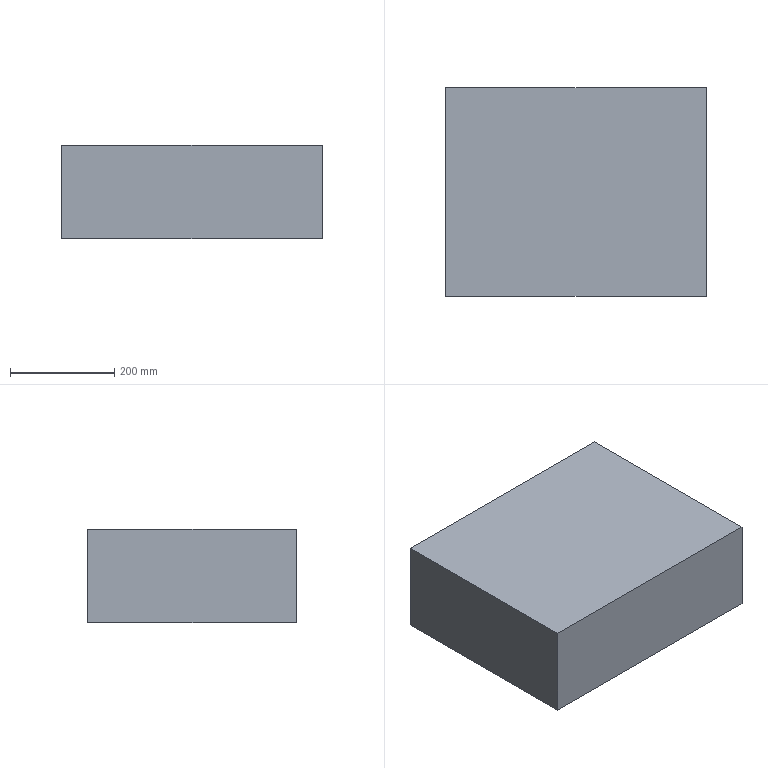Part | NX | features main panel 2 | 1 solid | 6 faces | box 500 x 400 x 180 mm | volume 36000000 mm3 | plane 6
STEP:
#1=CARTESIAN_POINT('',(250.,-600.,0.));
#2=VERTEX_POINT('',#1);
#3=CARTESIAN_POINT('',(-250.,-600.,0.));
#4=VERTEX_POINT('',#3);
#5=CARTESIAN_POINT('',(-250.,-600.,0.));
#6=DIRECTION('',(1.,0.,0.));
#7=VECTOR('',#6,1000.);
#8=LINE('',#5,#7);
#9=EDGE_CURVE('',#2,#4,#8,.F.);
#10=ORIENTED_EDGE('',*,*,#9,.F.);
#11=CARTESIAN_POINT('',(250.,-200.,0.));
#12=VERTEX_POINT('',#11);
#13=CARTESIAN_POINT('',(250.,-600.,0.));
#14=DIRECTION('',(0.,1.,0.));
#15=VECTOR('',#14,1000.);
#16=LINE('',#13,#15);
#17=EDGE_CURVE('',#12,#2,#16,.F.);
#18=ORIENTED_EDGE('',*,*,#17,.F.);
#19=CARTESIAN_POINT('',(-250.,-200.,0.));
#20=VERTEX_POINT('',#19);
#21=CARTESIAN_POINT('',(-250.,-200.,0.));
#22=DIRECTION('',(1.,0.,0.));
#23=VECTOR('',#22,1000.);
#24=LINE('',#21,#23);
#25=EDGE_CURVE('',#20,#12,#24,.T.);
#26=ORIENTED_EDGE('',*,*,#25,.F.);
#27=CARTESIAN_POINT('',(-250.,-600.,0.));
#28=DIRECTION('',(0.,1.,0.));
#29=VECTOR('',#28,1000.);
#30=LINE('',#27,#29);
#31=EDGE_CURVE('',#4,#20,#30,.T.);
#32=ORIENTED_EDGE('',*,*,#31,.F.);
#33=EDGE_LOOP('',(#10,#18,#26,#32));
#34=FACE_BOUND('',#33,.T.);
#35=CARTESIAN_POINT('',(-250.,-200.,0.));
#36=DIRECTION('',(0.,0.,-1.));
#37=DIRECTION('',(-1.,0.,0.));
#38=AXIS2_PLACEMENT_3D('',#35,#36,#37);
#39=PLANE('',#38);
#40=ADVANCED_FACE('',(#34),#39,.F.);
#41=CARTESIAN_POINT('',(-250.,-600.,-180.));
#42=VERTEX_POINT('',#41);
#43=CARTESIAN_POINT('',(-250.,-200.,-180.));
#44=VERTEX_POINT('',#43);
#45=CARTESIAN_POINT('',(-250.,-200.,-180.));
#46=DIRECTION('',(0.,1.,0.));
#47=VECTOR('',#46,1000.);
#48=LINE('',#45,#47);
#49=EDGE_CURVE('',#42,#44,#48,.T.);
#50=ORIENTED_EDGE('',*,*,#49,.F.);
#51=CARTESIAN_POINT('',(-250.,-600.,-180.));
#52=DIRECTION('',(0.,0.,-1.));
#53=VECTOR('',#52,1000.);
#54=LINE('',#51,#53);
#55=EDGE_CURVE('',#4,#42,#54,.T.);
#56=ORIENTED_EDGE('',*,*,#55,.F.);
#57=ORIENTED_EDGE('',*,*,#31,.T.);
#58=CARTESIAN_POINT('',(-250.,-200.,-180.));
#59=DIRECTION('',(0.,0.,1.));
#60=VECTOR('',#59,1000.);
#61=LINE('',#58,#60);
#62=EDGE_CURVE('',#44,#20,#61,.T.);
#63=ORIENTED_EDGE('',*,*,#62,.F.);
#64=EDGE_LOOP('',(#50,#56,#57,#63));
#65=FACE_BOUND('',#64,.T.);
#66=CARTESIAN_POINT('',(-250.,-600.,-180.));
#67=DIRECTION('',(-1.,0.,0.));
#68=DIRECTION('',(0.,0.,1.));
#69=AXIS2_PLACEMENT_3D('',#66,#67,#68);
#70=PLANE('',#69);
#71=ADVANCED_FACE('',(#65),#70,.T.);
#72=CARTESIAN_POINT('',(250.,-200.,-180.));
#73=VERTEX_POINT('',#72);
#74=CARTESIAN_POINT('',(-250.,-200.,-180.));
#75=DIRECTION('',(-1.,0.,0.));
#76=VECTOR('',#75,1000.);
#77=LINE('',#74,#76);
#78=EDGE_CURVE('',#44,#73,#77,.F.);
#79=ORIENTED_EDGE('',*,*,#78,.F.);
#80=ORIENTED_EDGE('',*,*,#62,.T.);
#81=ORIENTED_EDGE('',*,*,#25,.T.);
#82=CARTESIAN_POINT('',(250.,-200.,-180.));
#83=DIRECTION('',(0.,0.,-1.));
#84=VECTOR('',#83,1000.);
#85=LINE('',#82,#84);
#86=EDGE_CURVE('',#73,#12,#85,.F.);
#87=ORIENTED_EDGE('',*,*,#86,.F.);
#88=EDGE_LOOP('',(#79,#80,#81,#87));
#89=FACE_BOUND('',#88,.T.);
#90=CARTESIAN_POINT('',(-250.,-200.,-180.));
#91=DIRECTION('',(0.,1.,0.));
#92=DIRECTION('',(0.,0.,1.));
#93=AXIS2_PLACEMENT_3D('',#90,#91,#92);
#94=PLANE('',#93);
#95=ADVANCED_FACE('',(#89),#94,.T.);
#96=CARTESIAN_POINT('',(250.,-600.,-180.));
#97=VERTEX_POINT('',#96);
#98=CARTESIAN_POINT('',(250.,-200.,-180.));
#99=DIRECTION('',(0.,1.,0.));
#100=VECTOR('',#99,1000.);
#101=LINE('',#98,#100);
#102=EDGE_CURVE('',#73,#97,#101,.F.);
#103=ORIENTED_EDGE('',*,*,#102,.F.);
#104=ORIENTED_EDGE('',*,*,#86,.T.);
#105=ORIENTED_EDGE('',*,*,#17,.T.);
#106=CARTESIAN_POINT('',(250.,-600.,-180.));
#107=DIRECTION('',(0.,0.,-1.));
#108=VECTOR('',#107,1000.);
#109=LINE('',#106,#108);
#110=EDGE_CURVE('',#97,#2,#109,.F.);
#111=ORIENTED_EDGE('',*,*,#110,.F.);
#112=EDGE_LOOP('',(#103,#104,#105,#111));
#113=FACE_BOUND('',#112,.T.);
#114=CARTESIAN_POINT('',(250.,-600.,-180.));
#115=DIRECTION('',(1.,0.,0.));
#116=DIRECTION('',(0.,0.,-1.));
#117=AXIS2_PLACEMENT_3D('',#114,#115,#116);
#118=PLANE('',#117);
#119=ADVANCED_FACE('',(#113),#118,.T.);
#120=CARTESIAN_POINT('',(-250.,-600.,-180.));
#121=DIRECTION('',(-1.,0.,0.));
#122=VECTOR('',#121,1000.);
#123=LINE('',#120,#122);
#124=EDGE_CURVE('',#97,#42,#123,.T.);
#125=ORIENTED_EDGE('',*,*,#124,.F.);
#126=ORIENTED_EDGE('',*,*,#110,.T.);
#127=ORIENTED_EDGE('',*,*,#9,.T.);
#128=ORIENTED_EDGE('',*,*,#55,.T.);
#129=EDGE_LOOP('',(#125,#126,#127,#128));
#130=FACE_BOUND('',#129,.T.);
#131=CARTESIAN_POINT('',(-250.,-600.,-180.));
#132=DIRECTION('',(0.,-1.,0.));
#133=DIRECTION('',(0.,0.,-1.));
#134=AXIS2_PLACEMENT_3D('',#131,#132,#133);
#135=PLANE('',#134);
#136=ADVANCED_FACE('',(#130),#135,.T.);
#137=ORIENTED_EDGE('',*,*,#102,.T.);
#138=ORIENTED_EDGE('',*,*,#124,.T.);
#139=ORIENTED_EDGE('',*,*,#49,.T.);
#140=ORIENTED_EDGE('',*,*,#78,.T.);
#141=EDGE_LOOP('',(#137,#138,#139,#140));
#142=FACE_BOUND('',#141,.T.);
#143=CARTESIAN_POINT('',(-250.,-200.,-180.));
#144=DIRECTION('',(0.,0.,-1.));
#145=DIRECTION('',(-1.,0.,0.));
#146=AXIS2_PLACEMENT_3D('',#143,#144,#145);
#147=PLANE('',#146);
#148=ADVANCED_FACE('',(#142),#147,.T.);
#149=CLOSED_SHELL('',(#40,#71,#95,#119,#136,#148));
#150=MANIFOLD_SOLID_BREP('',#149);
#151=(LENGTH_UNIT()NAMED_UNIT(*)SI_UNIT(.MILLI.,.METRE.));
#152=UNCERTAINTY_MEASURE_WITH_UNIT(LENGTH_MEASURE(0.00001),#151,'','');
#153=(NAMED_UNIT(*)PLANE_ANGLE_UNIT()SI_UNIT($,.RADIAN.));
#154=(NAMED_UNIT(*)SI_UNIT($,.STERADIAN.)SOLID_ANGLE_UNIT());
#155=(GEOMETRIC_REPRESENTATION_CONTEXT(3)GLOBAL_UNCERTAINTY_ASSIGNED_CONTEXT((#152))GLOBAL_UNIT_ASSIGNED_CONTEXT((#151,#153,#154))REPRESENTATION_CONTEXT('',''));
#156=ADVANCED_BREP_SHAPE_REPRESENTATION('',(#150),#155);